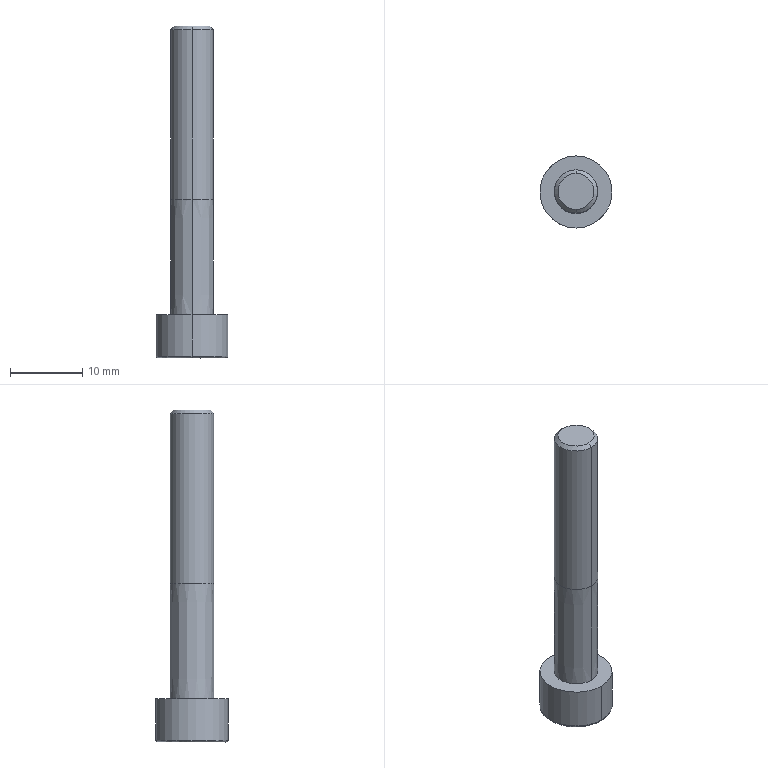Part | SolidWorks | features BaseBody 1 | 1 solid | 20 faces | box 10 x 10 x 46 mm | volume 1534 mm3 | plane 10 | cylinder 4 | cone 4 | spline 2 | commonest cylinder face diameters 6 x2 10 x2
STEP:
#1=CARTESIAN_POINT('',(591.518,-182.648,-27.862));
#2=VERTEX_POINT('',#1);
#3=CARTESIAN_POINT('',(591.54,-192.648,-27.862));
#4=VERTEX_POINT('',#3);
#5=CARTESIAN_POINT('',(591.54,-187.648,-27.862));
#6=DIRECTION('',(0.000000001,-0.000000003,1.));
#7=DIRECTION('',(0.,-1.,-0.000000003));
#8=AXIS2_PLACEMENT_3D('',#5,#6,#7);
#9=CIRCLE('',#8,5.);
#10=EDGE_CURVE('',#2,#4,#9,.T.);
#11=ORIENTED_EDGE('',*,*,#10,.F.);
#12=CARTESIAN_POINT('',(591.519,-182.898,-28.112));
#13=VERTEX_POINT('',#12);
#14=CARTESIAN_POINT('',(591.519,-182.898,-27.862));
#15=DIRECTION('',(-1.,-0.004352,0.000000001));
#16=DIRECTION('',(-0.004352,1.,0.000000003));
#17=AXIS2_PLACEMENT_3D('',#14,#15,#16);
#18=CIRCLE('',#17,0.25);
#19=EDGE_CURVE('',#2,#13,#18,.T.);
#20=ORIENTED_EDGE('',*,*,#19,.T.);
#21=CARTESIAN_POINT('',(591.561,-192.398,-28.112));
#22=VERTEX_POINT('',#21);
#23=CARTESIAN_POINT('',(591.519,-182.898,-28.112));
#24=CARTESIAN_POINT('',(582.019,-182.94,-28.112));
#25=CARTESIAN_POINT('',(582.061,-192.439,-28.112));
#26=CARTESIAN_POINT('',(591.561,-192.398,-28.112));
#27=(BOUNDED_CURVE()B_SPLINE_CURVE(3,(#23,#24,#25,#26),.UNSPECIFIED.,.F.,.F.)B_SPLINE_CURVE_WITH_KNOTS((4,4),(0.,1.),.UNSPECIFIED.)CURVE()GEOMETRIC_REPRESENTATION_ITEM()RATIONAL_B_SPLINE_CURVE((1.,0.3333,0.3333,1.))REPRESENTATION_ITEM(''));
#28=EDGE_CURVE('',#13,#22,#27,.T.);
#29=ORIENTED_EDGE('',*,*,#28,.T.);
#30=CARTESIAN_POINT('',(591.562,-192.648,-27.862));
#31=VERTEX_POINT('',#30);
#32=CARTESIAN_POINT('',(591.561,-192.398,-27.862));
#33=DIRECTION('',(1.,0.004352,-0.000000001));
#34=DIRECTION('',(0.004352,-1.,-0.000000003));
#35=AXIS2_PLACEMENT_3D('',#32,#33,#34);
#36=CIRCLE('',#35,0.25);
#37=EDGE_CURVE('',#31,#22,#36,.T.);
#38=ORIENTED_EDGE('',*,*,#37,.F.);
#39=CARTESIAN_POINT('',(591.54,-187.648,-27.862));
#40=DIRECTION('',(0.000000001,-0.000000003,1.));
#41=DIRECTION('',(0.,-1.,-0.000000003));
#42=AXIS2_PLACEMENT_3D('',#39,#40,#41);
#43=CIRCLE('',#42,5.);
#44=EDGE_CURVE('',#4,#31,#43,.T.);
#45=ORIENTED_EDGE('',*,*,#44,.F.);
#46=EDGE_LOOP('',(#11,#20,#29,#38,#45));
#47=FACE_OUTER_BOUND('',#46,.T.);
#48=CARTESIAN_POINT('',(591.518,-182.648,-27.862));
#49=CARTESIAN_POINT('',(581.518,-182.692,-27.862));
#50=CARTESIAN_POINT('',(581.562,-192.692,-27.862));
#51=CARTESIAN_POINT('',(591.562,-192.648,-27.862));
#52=CARTESIAN_POINT('',(591.518,-182.648,-28.008));
#53=CARTESIAN_POINT('',(581.518,-182.692,-28.008));
#54=CARTESIAN_POINT('',(581.562,-192.692,-28.008));
#55=CARTESIAN_POINT('',(591.562,-192.648,-28.008));
#56=CARTESIAN_POINT('',(591.519,-182.752,-28.112));
#57=CARTESIAN_POINT('',(581.726,-182.794,-28.112));
#58=CARTESIAN_POINT('',(581.768,-192.587,-28.112));
#59=CARTESIAN_POINT('',(591.561,-192.545,-28.112));
#60=CARTESIAN_POINT('',(591.519,-182.898,-28.112));
#61=CARTESIAN_POINT('',(582.019,-182.94,-28.112));
#62=CARTESIAN_POINT('',(582.061,-192.439,-28.112));
#63=CARTESIAN_POINT('',(591.561,-192.398,-28.112));
#64=(BOUNDED_SURFACE()B_SPLINE_SURFACE(3,3,((#48,#49,#50,#51),(#52,#53,#54,#55),(#56,#57,#58,#59),(#60,#61,#62,#63)),.UNSPECIFIED.,.F.,.F.,.F.)B_SPLINE_SURFACE_WITH_KNOTS((4,4),(4,4),(0.,1.),(0.,1.),.UNSPECIFIED.)GEOMETRIC_REPRESENTATION_ITEM()RATIONAL_B_SPLINE_SURFACE(((1.,0.3333,0.3333,1.),(0.8047,0.2682,0.2682,0.8047),(0.8047,0.2682,0.2682,0.8047),(1.,0.3333,0.3333,1.)))REPRESENTATION_ITEM('')SURFACE());
#65=ADVANCED_FACE('',(#47),#64,.T.);
#66=CARTESIAN_POINT('',(591.54,-190.648,-6.112));
#67=VERTEX_POINT('',#66);
#68=CARTESIAN_POINT('',(591.54,-184.648,-6.112));
#69=VERTEX_POINT('',#68);
#70=CARTESIAN_POINT('',(591.54,-187.648,-6.112));
#71=DIRECTION('',(0.000000001,-0.000000003,1.));
#72=DIRECTION('',(0.,-1.,-0.000000003));
#73=AXIS2_PLACEMENT_3D('',#70,#71,#72);
#74=CIRCLE('',#73,3.);
#75=EDGE_CURVE('',#67,#69,#74,.T.);
#76=ORIENTED_EDGE('',*,*,#75,.T.);
#77=CARTESIAN_POINT('',(591.54,-184.648,17.388));
#78=VERTEX_POINT('',#77);
#79=CARTESIAN_POINT('',(591.54,-184.648,5.638));
#80=DIRECTION('',(0.000000001,-0.000000003,1.));
#81=VECTOR('',#80,1000.);
#82=LINE('',#79,#81);
#83=EDGE_CURVE('',#69,#78,#82,.T.);
#84=ORIENTED_EDGE('',*,*,#83,.T.);
#85=CARTESIAN_POINT('',(591.54,-190.648,17.388));
#86=VERTEX_POINT('',#85);
#87=CARTESIAN_POINT('',(591.54,-187.648,17.388));
#88=DIRECTION('',(-0.000000001,0.000000003,-1.));
#89=DIRECTION('',(0.,-1.,-0.000000003));
#90=AXIS2_PLACEMENT_3D('',#87,#88,#89);
#91=CIRCLE('',#90,3.);
#92=EDGE_CURVE('',#78,#86,#91,.T.);
#93=ORIENTED_EDGE('',*,*,#92,.T.);
#94=CARTESIAN_POINT('',(591.54,-190.648,5.638));
#95=DIRECTION('',(0.000000001,-0.000000003,1.));
#96=VECTOR('',#95,1000.);
#97=LINE('',#94,#96);
#98=EDGE_CURVE('',#67,#86,#97,.T.);
#99=ORIENTED_EDGE('',*,*,#98,.F.);
#100=EDGE_LOOP('',(#76,#84,#93,#99));
#101=FACE_OUTER_BOUND('',#100,.T.);
#102=CARTESIAN_POINT('',(591.54,-187.648,5.638));
#103=DIRECTION('',(0.000000001,-0.000000003,1.));
#104=DIRECTION('',(0.,-1.,-0.000000003));
#105=AXIS2_PLACEMENT_3D('',#102,#103,#104);
#106=CYLINDRICAL_SURFACE('',#105,3.);
#107=ADVANCED_FACE('',(#101),#106,.T.);
#108=CARTESIAN_POINT('',(591.54,-190.647,-22.112));
#109=VERTEX_POINT('',#108);
#110=CARTESIAN_POINT('',(591.54,-184.65,-22.112));
#111=VERTEX_POINT('',#110);
#112=CARTESIAN_POINT('',(591.54,-187.648,-22.112));
#113=DIRECTION('',(0.000000001,-0.000000003,1.));
#114=DIRECTION('',(0.,-1.,-0.000000003));
#115=AXIS2_PLACEMENT_3D('',#112,#113,#114);
#116=CIRCLE('',#115,2.998);
#117=EDGE_CURVE('',#109,#111,#116,.T.);
#118=ORIENTED_EDGE('',*,*,#117,.T.);
#119=CARTESIAN_POINT('',(591.54,-184.648,-6.112));
#120=DIRECTION('',(0.000000001,0.00009375,1.));
#121=VECTOR('',#120,1000.);
#122=LINE('',#119,#121);
#123=EDGE_CURVE('',#111,#69,#122,.T.);
#124=ORIENTED_EDGE('',*,*,#123,.T.);
#125=ORIENTED_EDGE('',*,*,#75,.F.);
#126=CARTESIAN_POINT('',(591.54,-190.648,-6.112));
#127=DIRECTION('',(0.000000001,-0.00009375,1.));
#128=VECTOR('',#127,1000.);
#129=LINE('',#126,#128);
#130=EDGE_CURVE('',#109,#67,#129,.T.);
#131=ORIENTED_EDGE('',*,*,#130,.F.);
#132=EDGE_LOOP('',(#118,#124,#125,#131));
#133=FACE_OUTER_BOUND('',#132,.T.);
#134=CARTESIAN_POINT('',(591.54,-187.648,-6.112));
#135=DIRECTION('',(0.000000001,-0.000000003,1.));
#136=DIRECTION('',(0.,-1.,-0.000000003));
#137=AXIS2_PLACEMENT_3D('',#134,#135,#136);
#138=CONICAL_SURFACE('',#137,3.,0.00009375);
#139=ADVANCED_FACE('',(#133),#138,.T.);
#140=CARTESIAN_POINT('',(591.54,-185.148,17.888));
#141=VERTEX_POINT('',#140);
#142=CARTESIAN_POINT('',(591.54,-190.148,17.888));
#143=VERTEX_POINT('',#142);
#144=CARTESIAN_POINT('',(591.54,-187.648,17.888));
#145=DIRECTION('',(-0.000000001,0.000000003,-1.));
#146=DIRECTION('',(0.,1.,0.000000003));
#147=AXIS2_PLACEMENT_3D('',#144,#145,#146);
#148=CIRCLE('',#147,2.5);
#149=EDGE_CURVE('',#141,#143,#148,.T.);
#150=ORIENTED_EDGE('',*,*,#149,.T.);
#151=CARTESIAN_POINT('',(591.54,-190.648,17.388));
#152=DIRECTION('',(-0.000000001,-0.7071,-0.7071));
#153=VECTOR('',#152,1000.);
#154=LINE('',#151,#153);
#155=EDGE_CURVE('',#143,#86,#154,.T.);
#156=ORIENTED_EDGE('',*,*,#155,.T.);
#157=ORIENTED_EDGE('',*,*,#92,.F.);
#158=CARTESIAN_POINT('',(591.54,-184.648,17.388));
#159=DIRECTION('',(-0.000000001,0.7071,-0.7071));
#160=VECTOR('',#159,1000.);
#161=LINE('',#158,#160);
#162=EDGE_CURVE('',#141,#78,#161,.T.);
#163=ORIENTED_EDGE('',*,*,#162,.F.);
#164=EDGE_LOOP('',(#150,#156,#157,#163));
#165=FACE_OUTER_BOUND('',#164,.T.);
#166=CARTESIAN_POINT('',(591.54,-187.648,17.388));
#167=DIRECTION('',(-0.000000001,0.000000003,-1.));
#168=DIRECTION('',(0.,1.,0.000000003));
#169=AXIS2_PLACEMENT_3D('',#166,#167,#168);
#170=CONICAL_SURFACE('',#169,3.,0.7854);
#171=ADVANCED_FACE('',(#165),#170,.T.);
#172=ORIENTED_EDGE('',*,*,#44,.T.);
#173=CARTESIAN_POINT('',(591.54,-182.648,-27.862));
#174=VERTEX_POINT('',#173);
#175=CARTESIAN_POINT('',(591.54,-187.648,-27.862));
#176=DIRECTION('',(0.000000001,-0.000000003,1.));
#177=DIRECTION('',(0.,-1.,-0.000000003));
#178=AXIS2_PLACEMENT_3D('',#175,#176,#177);
#179=CIRCLE('',#178,5.);
#180=EDGE_CURVE('',#31,#174,#179,.T.);
#181=ORIENTED_EDGE('',*,*,#180,.T.);
#182=CARTESIAN_POINT('',(591.54,-182.648,-22.112));
#183=VERTEX_POINT('',#182);
#184=CARTESIAN_POINT('',(591.54,-182.648,-24.987));
#185=DIRECTION('',(0.000000001,-0.000000003,1.));
#186=VECTOR('',#185,1000.);
#187=LINE('',#184,#186);
#188=EDGE_CURVE('',#174,#183,#187,.T.);
#189=ORIENTED_EDGE('',*,*,#188,.T.);
#190=CARTESIAN_POINT('',(591.54,-192.648,-22.112));
#191=VERTEX_POINT('',#190);
#192=CARTESIAN_POINT('',(591.54,-187.648,-22.112));
#193=DIRECTION('',(0.000000001,-0.000000003,1.));
#194=DIRECTION('',(0.,-1.,-0.000000003));
#195=AXIS2_PLACEMENT_3D('',#192,#193,#194);
#196=CIRCLE('',#195,5.);
#197=EDGE_CURVE('',#191,#183,#196,.T.);
#198=ORIENTED_EDGE('',*,*,#197,.F.);
#199=CARTESIAN_POINT('',(591.54,-192.648,-24.987));
#200=DIRECTION('',(0.000000001,-0.000000003,1.));
#201=VECTOR('',#200,1000.);
#202=LINE('',#199,#201);
#203=EDGE_CURVE('',#4,#191,#202,.T.);
#204=ORIENTED_EDGE('',*,*,#203,.F.);
#205=EDGE_LOOP('',(#172,#181,#189,#198,#204));
#206=FACE_OUTER_BOUND('',#205,.T.);
#207=CARTESIAN_POINT('',(591.54,-187.648,-24.987));
#208=DIRECTION('',(0.000000001,-0.000000003,1.));
#209=DIRECTION('',(0.,-1.,-0.000000003));
#210=AXIS2_PLACEMENT_3D('',#207,#208,#209);
#211=CYLINDRICAL_SURFACE('',#210,5.);
#212=ADVANCED_FACE('',(#206),#211,.T.);
#213=ORIENTED_EDGE('',*,*,#83,.F.);
#214=CARTESIAN_POINT('',(591.54,-187.648,-6.112));
#215=DIRECTION('',(0.000000001,-0.000000003,1.));
#216=DIRECTION('',(0.,-1.,-0.000000003));
#217=AXIS2_PLACEMENT_3D('',#214,#215,#216);
#218=CIRCLE('',#217,3.);
#219=EDGE_CURVE('',#69,#67,#218,.T.);
#220=ORIENTED_EDGE('',*,*,#219,.T.);
#221=ORIENTED_EDGE('',*,*,#98,.T.);
#222=CARTESIAN_POINT('',(591.54,-187.648,17.388));
#223=DIRECTION('',(-0.000000001,0.000000003,-1.));
#224=DIRECTION('',(0.,-1.,-0.000000003));
#225=AXIS2_PLACEMENT_3D('',#222,#223,#224);
#226=CIRCLE('',#225,3.);
#227=EDGE_CURVE('',#86,#78,#226,.T.);
#228=ORIENTED_EDGE('',*,*,#227,.T.);
#229=EDGE_LOOP('',(#213,#220,#221,#228));
#230=FACE_OUTER_BOUND('',#229,.T.);
#231=CARTESIAN_POINT('',(591.54,-187.648,5.638));
#232=DIRECTION('',(0.000000001,-0.000000003,1.));
#233=DIRECTION('',(0.,-1.,-0.000000003));
#234=AXIS2_PLACEMENT_3D('',#231,#232,#233);
#235=CYLINDRICAL_SURFACE('',#234,3.);
#236=ADVANCED_FACE('',(#230),#235,.T.);
#237=ORIENTED_EDGE('',*,*,#123,.F.);
#238=CARTESIAN_POINT('',(591.54,-187.648,-22.112));
#239=DIRECTION('',(0.000000001,-0.000000003,1.));
#240=DIRECTION('',(0.,-1.,-0.000000003));
#241=AXIS2_PLACEMENT_3D('',#238,#239,#240);
#242=CIRCLE('',#241,2.998);
#243=EDGE_CURVE('',#111,#109,#242,.T.);
#244=ORIENTED_EDGE('',*,*,#243,.T.);
#245=ORIENTED_EDGE('',*,*,#130,.T.);
#246=ORIENTED_EDGE('',*,*,#219,.F.);
#247=EDGE_LOOP('',(#237,#244,#245,#246));
#248=FACE_OUTER_BOUND('',#247,.T.);
#249=CARTESIAN_POINT('',(591.54,-187.648,-6.112));
#250=DIRECTION('',(0.000000001,-0.000000003,1.));
#251=DIRECTION('',(0.,-1.,-0.000000003));
#252=AXIS2_PLACEMENT_3D('',#249,#250,#251);
#253=CONICAL_SURFACE('',#252,3.,0.00009375);
#254=ADVANCED_FACE('',(#248),#253,.T.);
#255=ORIENTED_EDGE('',*,*,#155,.F.);
#256=CARTESIAN_POINT('',(591.54,-187.648,17.888));
#257=DIRECTION('',(-0.000000001,0.000000003,-1.));
#258=DIRECTION('',(0.,1.,0.000000003));
#259=AXIS2_PLACEMENT_3D('',#256,#257,#258);
#260=CIRCLE('',#259,2.5);
#261=EDGE_CURVE('',#143,#141,#260,.T.);
#262=ORIENTED_EDGE('',*,*,#261,.T.);
#263=ORIENTED_EDGE('',*,*,#162,.T.);
#264=ORIENTED_EDGE('',*,*,#227,.F.);
#265=EDGE_LOOP('',(#255,#262,#263,#264));
#266=FACE_OUTER_BOUND('',#265,.T.);
#267=CARTESIAN_POINT('',(591.54,-187.648,17.388));
#268=DIRECTION('',(-0.000000001,0.000000003,-1.));
#269=DIRECTION('',(0.,1.,0.000000003));
#270=AXIS2_PLACEMENT_3D('',#267,#268,#269);
#271=CONICAL_SURFACE('',#270,3.,0.7854);
#272=ADVANCED_FACE('',(#266),#271,.T.);
#273=ORIENTED_EDGE('',*,*,#117,.F.);
#274=ORIENTED_EDGE('',*,*,#243,.F.);
#275=EDGE_LOOP('',(#273,#274));
#276=FACE_BOUND('',#275,.T.);
#277=ORIENTED_EDGE('',*,*,#197,.T.);
#278=CARTESIAN_POINT('',(591.54,-187.648,-22.112));
#279=DIRECTION('',(0.000000001,-0.000000003,1.));
#280=DIRECTION('',(0.,-1.,-0.000000003));
#281=AXIS2_PLACEMENT_3D('',#278,#279,#280);
#282=CIRCLE('',#281,5.);
#283=EDGE_CURVE('',#183,#191,#282,.T.);
#284=ORIENTED_EDGE('',*,*,#283,.T.);
#285=EDGE_LOOP('',(#277,#284));
#286=FACE_OUTER_BOUND('',#285,.T.);
#287=CARTESIAN_POINT('',(591.551,-190.148,-22.112));
#288=DIRECTION('',(0.000000001,-0.000000003,1.));
#289=DIRECTION('',(0.,-1.,-0.000000003));
#290=AXIS2_PLACEMENT_3D('',#287,#288,#289);
#291=PLANE('',#290);
#292=ADVANCED_FACE('',(#276,#286),#291,.T.);
#293=ORIENTED_EDGE('',*,*,#149,.F.);
#294=ORIENTED_EDGE('',*,*,#261,.F.);
#295=EDGE_LOOP('',(#293,#294));
#296=FACE_OUTER_BOUND('',#295,.T.);
#297=CARTESIAN_POINT('',(591.545,-188.898,17.888));
#298=DIRECTION('',(0.000000001,-0.000000003,1.));
#299=DIRECTION('',(0.,-1.,-0.000000003));
#300=AXIS2_PLACEMENT_3D('',#297,#298,#299);
#301=PLANE('',#300);
#302=ADVANCED_FACE('',(#296),#301,.T.);
#303=ORIENTED_EDGE('',*,*,#188,.F.);
#304=CARTESIAN_POINT('',(591.54,-187.648,-27.862));
#305=DIRECTION('',(0.000000001,-0.000000003,1.));
#306=DIRECTION('',(0.,-1.,-0.000000003));
#307=AXIS2_PLACEMENT_3D('',#304,#305,#306);
#308=CIRCLE('',#307,5.);
#309=EDGE_CURVE('',#174,#2,#308,.T.);
#310=ORIENTED_EDGE('',*,*,#309,.T.);
#311=ORIENTED_EDGE('',*,*,#10,.T.);
#312=ORIENTED_EDGE('',*,*,#203,.T.);
#313=ORIENTED_EDGE('',*,*,#283,.F.);
#314=EDGE_LOOP('',(#303,#310,#311,#312,#313));
#315=FACE_OUTER_BOUND('',#314,.T.);
#316=CARTESIAN_POINT('',(591.54,-187.648,-24.987));
#317=DIRECTION('',(0.000000001,-0.000000003,1.));
#318=DIRECTION('',(0.,-1.,-0.000000003));
#319=AXIS2_PLACEMENT_3D('',#316,#317,#318);
#320=CYLINDRICAL_SURFACE('',#319,5.);
#321=ADVANCED_FACE('',(#315),#320,.T.);
#322=ORIENTED_EDGE('',*,*,#19,.F.);
#323=ORIENTED_EDGE('',*,*,#309,.F.);
#324=ORIENTED_EDGE('',*,*,#180,.F.);
#325=ORIENTED_EDGE('',*,*,#37,.T.);
#326=CARTESIAN_POINT('',(591.561,-192.398,-28.112));
#327=CARTESIAN_POINT('',(601.061,-192.357,-28.112));
#328=CARTESIAN_POINT('',(601.019,-182.857,-28.112));
#329=CARTESIAN_POINT('',(591.519,-182.898,-28.112));
#330=(BOUNDED_CURVE()B_SPLINE_CURVE(3,(#326,#327,#328,#329),.UNSPECIFIED.,.F.,.T.)B_SPLINE_CURVE_WITH_KNOTS((4,4),(0.,1.),.UNSPECIFIED.)CURVE()GEOMETRIC_REPRESENTATION_ITEM()RATIONAL_B_SPLINE_CURVE((1.,0.3333,0.3333,1.))REPRESENTATION_ITEM(''));
#331=EDGE_CURVE('',#22,#13,#330,.T.);
#332=ORIENTED_EDGE('',*,*,#331,.T.);
#333=EDGE_LOOP('',(#322,#323,#324,#325,#332));
#334=FACE_OUTER_BOUND('',#333,.T.);
#335=CARTESIAN_POINT('',(591.562,-192.648,-27.862));
#336=CARTESIAN_POINT('',(601.562,-192.605,-27.862));
#337=CARTESIAN_POINT('',(601.518,-182.605,-27.862));
#338=CARTESIAN_POINT('',(591.518,-182.648,-27.862));
#339=CARTESIAN_POINT('',(591.562,-192.648,-28.008));
#340=CARTESIAN_POINT('',(601.562,-192.605,-28.008));
#341=CARTESIAN_POINT('',(601.518,-182.605,-28.008));
#342=CARTESIAN_POINT('',(591.518,-182.648,-28.008));
#343=CARTESIAN_POINT('',(591.561,-192.545,-28.112));
#344=CARTESIAN_POINT('',(601.354,-192.502,-28.112));
#345=CARTESIAN_POINT('',(601.311,-182.709,-28.112));
#346=CARTESIAN_POINT('',(591.519,-182.752,-28.112));
#347=CARTESIAN_POINT('',(591.561,-192.398,-28.112));
#348=CARTESIAN_POINT('',(601.061,-192.357,-28.112));
#349=CARTESIAN_POINT('',(601.019,-182.857,-28.112));
#350=CARTESIAN_POINT('',(591.519,-182.898,-28.112));
#351=(BOUNDED_SURFACE()B_SPLINE_SURFACE(3,3,((#335,#336,#337,#338),(#339,#340,#341,#342),(#343,#344,#345,#346),(#347,#348,#349,#350)),.UNSPECIFIED.,.F.,.F.,.F.)B_SPLINE_SURFACE_WITH_KNOTS((4,4),(4,4),(0.,1.),(0.,1.),.UNSPECIFIED.)GEOMETRIC_REPRESENTATION_ITEM()RATIONAL_B_SPLINE_SURFACE(((1.,0.3333,0.3333,1.),(0.8047,0.2682,0.2682,0.8047),(0.8047,0.2682,0.2682,0.8047),(1.,0.3333,0.3333,1.)))REPRESENTATION_ITEM('')SURFACE());
#352=ADVANCED_FACE('',(#334),#351,.T.);
#353=ORIENTED_EDGE('',*,*,#28,.F.);
#354=ORIENTED_EDGE('',*,*,#331,.F.);
#355=EDGE_LOOP('',(#353,#354));
#356=FACE_OUTER_BOUND('',#355,.T.);
#357=CARTESIAN_POINT('',(594.034,-186.194,-28.112));
#358=VERTEX_POINT('',#357);
#359=CARTESIAN_POINT('',(591.527,-184.761,-28.112));
#360=VERTEX_POINT('',#359);
#361=CARTESIAN_POINT('',(594.034,-186.194,-28.112));
#362=DIRECTION('',(-0.8682,0.4962,0.000000002));
#363=VECTOR('',#362,1000.);
#364=LINE('',#361,#363);
#365=EDGE_CURVE('',#358,#360,#364,.T.);
#366=ORIENTED_EDGE('',*,*,#365,.T.);
#367=CARTESIAN_POINT('',(589.034,-186.216,-28.112));
#368=VERTEX_POINT('',#367);
#369=CARTESIAN_POINT('',(591.527,-184.761,-28.112));
#370=DIRECTION('',(-0.8638,-0.5038,-0.000000001));
#371=VECTOR('',#370,1000.);
#372=LINE('',#369,#371);
#373=EDGE_CURVE('',#360,#368,#372,.T.);
#374=ORIENTED_EDGE('',*,*,#373,.T.);
#375=CARTESIAN_POINT('',(589.046,-189.102,-28.112));
#376=VERTEX_POINT('',#375);
#377=CARTESIAN_POINT('',(589.034,-186.216,-28.112));
#378=DIRECTION('',(0.004352,-1.,-0.000000003));
#379=VECTOR('',#378,1000.);
#380=LINE('',#377,#379);
#381=EDGE_CURVE('',#368,#376,#380,.T.);
#382=ORIENTED_EDGE('',*,*,#381,.T.);
#383=CARTESIAN_POINT('',(591.553,-190.535,-28.112));
#384=VERTEX_POINT('',#383);
#385=CARTESIAN_POINT('',(589.046,-189.102,-28.112));
#386=DIRECTION('',(0.8682,-0.4962,-0.000000002));
#387=VECTOR('',#386,1000.);
#388=LINE('',#385,#387);
#389=EDGE_CURVE('',#376,#384,#388,.T.);
#390=ORIENTED_EDGE('',*,*,#389,.T.);
#391=CARTESIAN_POINT('',(594.046,-189.081,-28.112));
#392=VERTEX_POINT('',#391);
#393=CARTESIAN_POINT('',(591.553,-190.535,-28.112));
#394=DIRECTION('',(0.8638,0.5038,0.000000001));
#395=VECTOR('',#394,1000.);
#396=LINE('',#393,#395);
#397=EDGE_CURVE('',#384,#392,#396,.T.);
#398=ORIENTED_EDGE('',*,*,#397,.T.);
#399=CARTESIAN_POINT('',(594.046,-189.081,-28.112));
#400=DIRECTION('',(-0.004352,1.,0.000000003));
#401=VECTOR('',#400,1000.);
#402=LINE('',#399,#401);
#403=EDGE_CURVE('',#392,#358,#402,.T.);
#404=ORIENTED_EDGE('',*,*,#403,.T.);
#405=EDGE_LOOP('',(#366,#374,#382,#390,#398,#404));
#406=FACE_BOUND('',#405,.T.);
#407=CARTESIAN_POINT('',(591.55,-190.023,-28.112));
#408=DIRECTION('',(-0.000000001,0.000000003,-1.));
#409=DIRECTION('',(0.,1.,0.000000003));
#410=AXIS2_PLACEMENT_3D('',#407,#408,#409);
#411=PLANE('',#410);
#412=ADVANCED_FACE('',(#356,#406),#411,.T.);
#413=CARTESIAN_POINT('',(589.034,-186.216,-25.112));
#414=VERTEX_POINT('',#413);
#415=CARTESIAN_POINT('',(589.034,-186.216,-28.112));
#416=DIRECTION('',(0.000000002,-0.000000003,1.));
#417=VECTOR('',#416,1000.);
#418=LINE('',#415,#417);
#419=EDGE_CURVE('',#368,#414,#418,.T.);
#420=ORIENTED_EDGE('',*,*,#419,.F.);
#421=ORIENTED_EDGE('',*,*,#373,.F.);
#422=CARTESIAN_POINT('',(591.527,-184.761,-25.112));
#423=VERTEX_POINT('',#422);
#424=CARTESIAN_POINT('',(591.527,-184.761,-28.112));
#425=DIRECTION('',(-0.000000002,0.000000003,-1.));
#426=VECTOR('',#425,1000.);
#427=LINE('',#424,#426);
#428=EDGE_CURVE('',#423,#360,#427,.T.);
#429=ORIENTED_EDGE('',*,*,#428,.F.);
#430=CARTESIAN_POINT('',(589.034,-186.216,-25.112));
#431=DIRECTION('',(0.8638,0.5038,0.));
#432=VECTOR('',#431,1000.);
#433=LINE('',#430,#432);
#434=EDGE_CURVE('',#414,#423,#433,.T.);
#435=ORIENTED_EDGE('',*,*,#434,.F.);
#436=EDGE_LOOP('',(#420,#421,#429,#435));
#437=FACE_OUTER_BOUND('',#436,.T.);
#438=CARTESIAN_POINT('',(589.034,-186.216,-28.112));
#439=DIRECTION('',(-0.5038,0.8638,0.000000003));
#440=DIRECTION('',(-0.8638,-0.5038,0.));
#441=AXIS2_PLACEMENT_3D('',#438,#439,#440);
#442=PLANE('',#441);
#443=ADVANCED_FACE('',(#437),#442,.F.);
#444=ORIENTED_EDGE('',*,*,#428,.T.);
#445=ORIENTED_EDGE('',*,*,#365,.F.);
#446=CARTESIAN_POINT('',(594.034,-186.194,-25.112));
#447=VERTEX_POINT('',#446);
#448=CARTESIAN_POINT('',(594.034,-186.194,-28.112));
#449=DIRECTION('',(0.000000001,0.000000002,-1.));
#450=VECTOR('',#449,1000.);
#451=LINE('',#448,#450);
#452=EDGE_CURVE('',#447,#358,#451,.T.);
#453=ORIENTED_EDGE('',*,*,#452,.F.);
#454=CARTESIAN_POINT('',(591.527,-184.761,-25.112));
#455=DIRECTION('',(0.8682,-0.4962,0.));
#456=VECTOR('',#455,1000.);
#457=LINE('',#454,#456);
#458=EDGE_CURVE('',#423,#447,#457,.T.);
#459=ORIENTED_EDGE('',*,*,#458,.F.);
#460=EDGE_LOOP('',(#444,#445,#453,#459));
#461=FACE_OUTER_BOUND('',#460,.T.);
#462=CARTESIAN_POINT('',(591.527,-184.761,-28.112));
#463=DIRECTION('',(0.4962,0.8682,0.000000003));
#464=DIRECTION('',(-0.8682,0.4962,0.));
#465=AXIS2_PLACEMENT_3D('',#462,#463,#464);
#466=PLANE('',#465);
#467=ADVANCED_FACE('',(#461),#466,.F.);
#468=ORIENTED_EDGE('',*,*,#452,.T.);
#469=ORIENTED_EDGE('',*,*,#403,.F.);
#470=CARTESIAN_POINT('',(594.046,-189.081,-25.112));
#471=VERTEX_POINT('',#470);
#472=CARTESIAN_POINT('',(594.046,-189.081,-28.112));
#473=DIRECTION('',(-0.000000001,0.,-1.));
#474=VECTOR('',#473,1000.);
#475=LINE('',#472,#474);
#476=EDGE_CURVE('',#471,#392,#475,.T.);
#477=ORIENTED_EDGE('',*,*,#476,.F.);
#478=CARTESIAN_POINT('',(594.034,-186.194,-25.112));
#479=DIRECTION('',(0.004352,-1.,0.));
#480=VECTOR('',#479,1000.);
#481=LINE('',#478,#480);
#482=EDGE_CURVE('',#447,#471,#481,.T.);
#483=ORIENTED_EDGE('',*,*,#482,.F.);
#484=EDGE_LOOP('',(#468,#469,#477,#483));
#485=FACE_OUTER_BOUND('',#484,.T.);
#486=CARTESIAN_POINT('',(594.034,-186.194,-28.112));
#487=DIRECTION('',(1.,0.004352,-0.000000001));
#488=DIRECTION('',(-0.004352,1.,0.));
#489=AXIS2_PLACEMENT_3D('',#486,#487,#488);
#490=PLANE('',#489);
#491=ADVANCED_FACE('',(#485),#490,.F.);
#492=ORIENTED_EDGE('',*,*,#476,.T.);
#493=ORIENTED_EDGE('',*,*,#397,.F.);
#494=CARTESIAN_POINT('',(591.553,-190.535,-25.112));
#495=VERTEX_POINT('',#494);
#496=CARTESIAN_POINT('',(591.553,-190.535,-28.112));
#497=DIRECTION('',(-0.000000002,0.000000003,-1.));
#498=VECTOR('',#497,1000.);
#499=LINE('',#496,#498);
#500=EDGE_CURVE('',#495,#384,#499,.T.);
#501=ORIENTED_EDGE('',*,*,#500,.F.);
#502=CARTESIAN_POINT('',(594.046,-189.081,-25.112));
#503=DIRECTION('',(-0.8638,-0.5038,0.));
#504=VECTOR('',#503,1000.);
#505=LINE('',#502,#504);
#506=EDGE_CURVE('',#471,#495,#505,.T.);
#507=ORIENTED_EDGE('',*,*,#506,.F.);
#508=EDGE_LOOP('',(#492,#493,#501,#507));
#509=FACE_OUTER_BOUND('',#508,.T.);
#510=CARTESIAN_POINT('',(594.046,-189.081,-28.112));
#511=DIRECTION('',(0.5038,-0.8638,-0.000000003));
#512=DIRECTION('',(0.8638,0.5038,0.));
#513=AXIS2_PLACEMENT_3D('',#510,#511,#512);
#514=PLANE('',#513);
#515=ADVANCED_FACE('',(#509),#514,.F.);
#516=ORIENTED_EDGE('',*,*,#500,.T.);
#517=ORIENTED_EDGE('',*,*,#389,.F.);
#518=CARTESIAN_POINT('',(589.046,-189.102,-25.112));
#519=VERTEX_POINT('',#518);
#520=CARTESIAN_POINT('',(589.046,-189.102,-28.112));
#521=DIRECTION('',(0.000000001,0.000000002,-1.));
#522=VECTOR('',#521,1000.);
#523=LINE('',#520,#522);
#524=EDGE_CURVE('',#519,#376,#523,.T.);
#525=ORIENTED_EDGE('',*,*,#524,.F.);
#526=CARTESIAN_POINT('',(591.553,-190.535,-25.112));
#527=DIRECTION('',(-0.8682,0.4962,0.));
#528=VECTOR('',#527,1000.);
#529=LINE('',#526,#528);
#530=EDGE_CURVE('',#495,#519,#529,.T.);
#531=ORIENTED_EDGE('',*,*,#530,.F.);
#532=EDGE_LOOP('',(#516,#517,#525,#531));
#533=FACE_OUTER_BOUND('',#532,.T.);
#534=CARTESIAN_POINT('',(591.553,-190.535,-28.112));
#535=DIRECTION('',(-0.4962,-0.8682,-0.000000003));
#536=DIRECTION('',(0.8682,-0.4962,0.));
#537=AXIS2_PLACEMENT_3D('',#534,#535,#536);
#538=PLANE('',#537);
#539=ADVANCED_FACE('',(#533),#538,.F.);
#540=ORIENTED_EDGE('',*,*,#524,.T.);
#541=ORIENTED_EDGE('',*,*,#381,.F.);
#542=ORIENTED_EDGE('',*,*,#419,.T.);
#543=CARTESIAN_POINT('',(589.046,-189.102,-25.112));
#544=DIRECTION('',(-0.004352,1.,0.));
#545=VECTOR('',#544,1000.);
#546=LINE('',#543,#545);
#547=EDGE_CURVE('',#519,#414,#546,.T.);
#548=ORIENTED_EDGE('',*,*,#547,.F.);
#549=EDGE_LOOP('',(#540,#541,#542,#548));
#550=FACE_OUTER_BOUND('',#549,.T.);
#551=CARTESIAN_POINT('',(589.046,-189.102,-28.112));
#552=DIRECTION('',(-1.,-0.004352,0.000000001));
#553=DIRECTION('',(0.004352,-1.,0.));
#554=AXIS2_PLACEMENT_3D('',#551,#552,#553);
#555=PLANE('',#554);
#556=ADVANCED_FACE('',(#550),#555,.F.);
#557=ORIENTED_EDGE('',*,*,#506,.T.);
#558=ORIENTED_EDGE('',*,*,#530,.T.);
#559=ORIENTED_EDGE('',*,*,#547,.T.);
#560=ORIENTED_EDGE('',*,*,#434,.T.);
#561=ORIENTED_EDGE('',*,*,#458,.T.);
#562=ORIENTED_EDGE('',*,*,#482,.T.);
#563=EDGE_LOOP('',(#557,#558,#559,#560,#561,#562));
#564=FACE_OUTER_BOUND('',#563,.T.);
#565=CARTESIAN_POINT('',(591.54,-187.648,-25.112));
#566=DIRECTION('',(-0.000000001,0.000000003,-1.));
#567=DIRECTION('',(0.,1.,0.000000003));
#568=AXIS2_PLACEMENT_3D('',#565,#566,#567);
#569=PLANE('',#568);
#570=ADVANCED_FACE('',(#564),#569,.T.);
#571=CLOSED_SHELL('',(#65,#107,#139,#171,#212,#236,#254,#272,#292,#302,#321,#352,#412,#443,#467,#491,#515,#539,#556,#570));
#572=MANIFOLD_SOLID_BREP('',#571);
#573=CARTESIAN_POINT('',(0.,0.,0.));
#574=DIRECTION('',(0.,0.,1.));
#575=DIRECTION('',(1.,0.,0.));
#576=AXIS2_PLACEMENT_3D('',#573,#574,#575);
#577=(LENGTH_UNIT()NAMED_UNIT(*)SI_UNIT(.MILLI.,.METRE.));
#578=UNCERTAINTY_MEASURE_WITH_UNIT(LENGTH_MEASURE(0.00001),#577,'','');
#579=(NAMED_UNIT(*)PLANE_ANGLE_UNIT()SI_UNIT($,.RADIAN.));
#580=(NAMED_UNIT(*)SI_UNIT($,.STERADIAN.)SOLID_ANGLE_UNIT());
#581=(GEOMETRIC_REPRESENTATION_CONTEXT(3)GLOBAL_UNCERTAINTY_ASSIGNED_CONTEXT((#578))GLOBAL_UNIT_ASSIGNED_CONTEXT((#577,#579,#580))REPRESENTATION_CONTEXT('',''));
#582=ADVANCED_BREP_SHAPE_REPRESENTATION('',(#572,#576),#581);